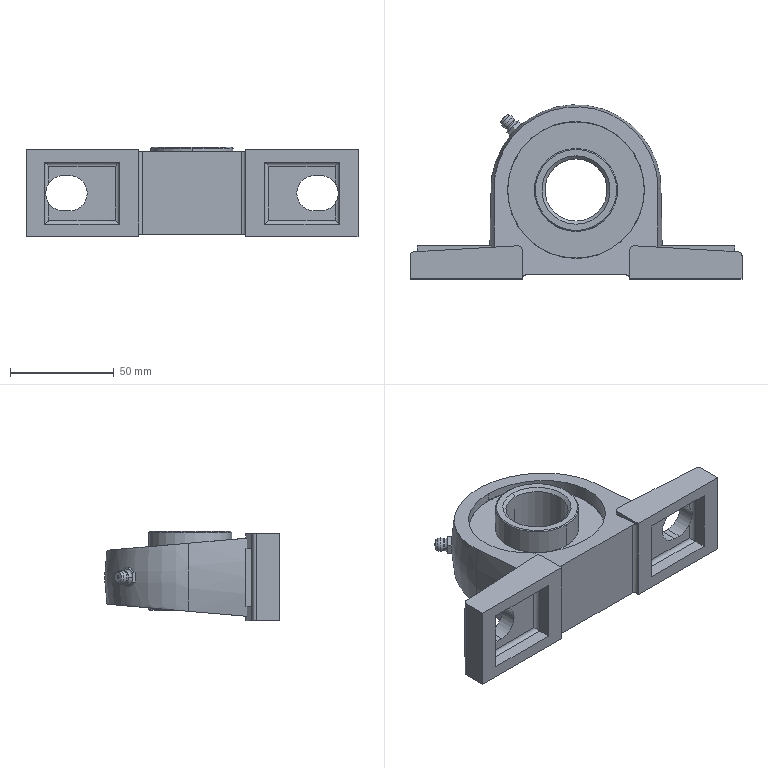Part | STEP file | ucp206_01V11 | 1 solid | 121 faces | box 160 x 84 x 43.2 mm | volume 181107 mm3 | plane 56 | cylinder 36 | cone 17 | torus 8 | sphere 3 | other 1 | commonest cylinder face diameters 4 x16 17 x6 40.1 x4 66 x4 6 x2 30 x2